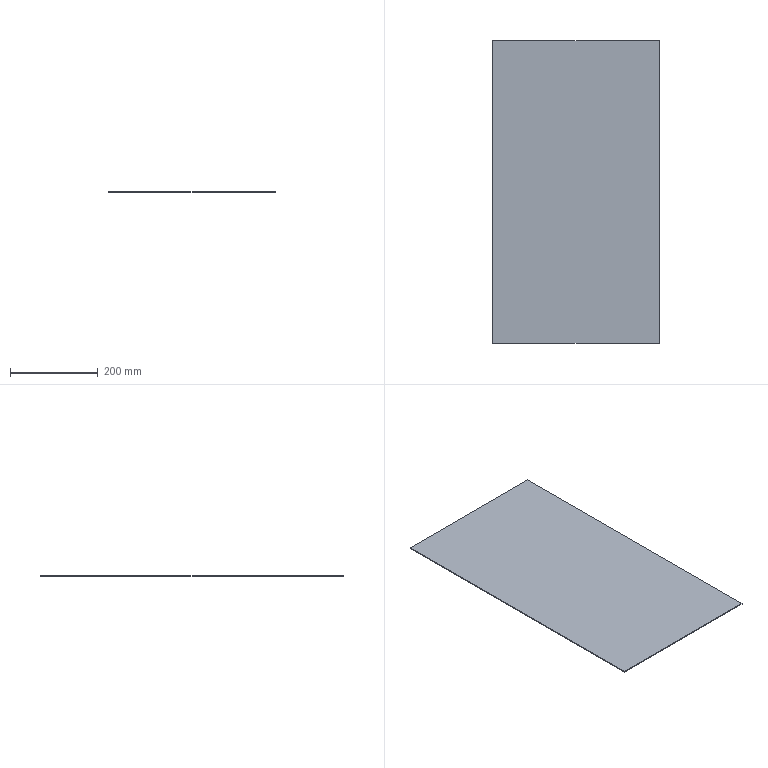Part | SolidWorks | features Extrusion 1 | 1 solid | 6 faces | box 380 x 690 x 2 mm | volume 524400 mm3 | plane 6
STEP:
#1=CARTESIAN_POINT('',(-337.882,161.453,0.));
#2=VERTEX_POINT('',#1);
#3=CARTESIAN_POINT('',(-337.882,-528.547,0.));
#4=VERTEX_POINT('',#3);
#5=CARTESIAN_POINT('',(-337.882,161.453,0.));
#6=DIRECTION('',(0.,-1.,0.));
#7=VECTOR('',#6,1000.);
#8=LINE('',#5,#7);
#9=EDGE_CURVE('',#2,#4,#8,.T.);
#10=ORIENTED_EDGE('',*,*,#9,.T.);
#11=CARTESIAN_POINT('',(-337.882,-528.547,2.));
#12=VERTEX_POINT('',#11);
#13=CARTESIAN_POINT('',(-337.882,-528.547,2.));
#14=DIRECTION('',(0.,0.,-1.));
#15=VECTOR('',#14,1000.);
#16=LINE('',#13,#15);
#17=EDGE_CURVE('',#12,#4,#16,.T.);
#18=ORIENTED_EDGE('',*,*,#17,.F.);
#19=CARTESIAN_POINT('',(-337.882,161.453,2.));
#20=VERTEX_POINT('',#19);
#21=CARTESIAN_POINT('',(-337.882,161.453,2.));
#22=DIRECTION('',(0.,-1.,0.));
#23=VECTOR('',#22,1000.);
#24=LINE('',#21,#23);
#25=EDGE_CURVE('',#20,#12,#24,.T.);
#26=ORIENTED_EDGE('',*,*,#25,.F.);
#27=CARTESIAN_POINT('',(-337.882,161.453,2.));
#28=DIRECTION('',(0.,0.,-1.));
#29=VECTOR('',#28,1000.);
#30=LINE('',#27,#29);
#31=EDGE_CURVE('',#20,#2,#30,.T.);
#32=ORIENTED_EDGE('',*,*,#31,.T.);
#33=EDGE_LOOP('',(#10,#18,#26,#32));
#34=FACE_OUTER_BOUND('',#33,.T.);
#35=CARTESIAN_POINT('',(-337.882,161.453,2.));
#36=DIRECTION('',(1.,0.,0.));
#37=DIRECTION('',(0.,1.,0.));
#38=AXIS2_PLACEMENT_3D('',#35,#36,#37);
#39=PLANE('',#38);
#40=ADVANCED_FACE('',(#34),#39,.F.);
#41=CARTESIAN_POINT('',(42.118,-528.547,0.));
#42=VERTEX_POINT('',#41);
#43=CARTESIAN_POINT('',(-337.882,-528.547,0.));
#44=DIRECTION('',(1.,0.,0.));
#45=VECTOR('',#44,1000.);
#46=LINE('',#43,#45);
#47=EDGE_CURVE('',#4,#42,#46,.T.);
#48=ORIENTED_EDGE('',*,*,#47,.T.);
#49=CARTESIAN_POINT('',(42.118,-528.547,2.));
#50=VERTEX_POINT('',#49);
#51=CARTESIAN_POINT('',(42.118,-528.547,2.));
#52=DIRECTION('',(0.,0.,-1.));
#53=VECTOR('',#52,1000.);
#54=LINE('',#51,#53);
#55=EDGE_CURVE('',#50,#42,#54,.T.);
#56=ORIENTED_EDGE('',*,*,#55,.F.);
#57=CARTESIAN_POINT('',(-337.882,-528.547,2.));
#58=DIRECTION('',(1.,0.,0.));
#59=VECTOR('',#58,1000.);
#60=LINE('',#57,#59);
#61=EDGE_CURVE('',#12,#50,#60,.T.);
#62=ORIENTED_EDGE('',*,*,#61,.F.);
#63=ORIENTED_EDGE('',*,*,#17,.T.);
#64=EDGE_LOOP('',(#48,#56,#62,#63));
#65=FACE_OUTER_BOUND('',#64,.T.);
#66=CARTESIAN_POINT('',(-337.882,-528.547,2.));
#67=DIRECTION('',(0.,1.,0.));
#68=DIRECTION('',(0.,0.,1.));
#69=AXIS2_PLACEMENT_3D('',#66,#67,#68);
#70=PLANE('',#69);
#71=ADVANCED_FACE('',(#65),#70,.F.);
#72=CARTESIAN_POINT('',(42.118,161.453,0.));
#73=VERTEX_POINT('',#72);
#74=CARTESIAN_POINT('',(42.118,161.453,0.));
#75=DIRECTION('',(0.,1.,0.));
#76=VECTOR('',#75,1000.);
#77=LINE('',#74,#76);
#78=EDGE_CURVE('',#42,#73,#77,.T.);
#79=ORIENTED_EDGE('',*,*,#78,.T.);
#80=CARTESIAN_POINT('',(42.118,161.453,2.));
#81=VERTEX_POINT('',#80);
#82=CARTESIAN_POINT('',(42.118,161.453,2.));
#83=DIRECTION('',(0.,0.,-1.));
#84=VECTOR('',#83,1000.);
#85=LINE('',#82,#84);
#86=EDGE_CURVE('',#81,#73,#85,.T.);
#87=ORIENTED_EDGE('',*,*,#86,.F.);
#88=CARTESIAN_POINT('',(42.118,161.453,2.));
#89=DIRECTION('',(0.,1.,0.));
#90=VECTOR('',#89,1000.);
#91=LINE('',#88,#90);
#92=EDGE_CURVE('',#50,#81,#91,.T.);
#93=ORIENTED_EDGE('',*,*,#92,.F.);
#94=ORIENTED_EDGE('',*,*,#55,.T.);
#95=EDGE_LOOP('',(#79,#87,#93,#94));
#96=FACE_OUTER_BOUND('',#95,.T.);
#97=CARTESIAN_POINT('',(42.118,161.453,2.));
#98=DIRECTION('',(-1.,0.,0.));
#99=DIRECTION('',(0.,-1.,0.));
#100=AXIS2_PLACEMENT_3D('',#97,#98,#99);
#101=PLANE('',#100);
#102=ADVANCED_FACE('',(#96),#101,.F.);
#103=CARTESIAN_POINT('',(-337.882,161.453,0.));
#104=DIRECTION('',(-1.,0.,0.));
#105=VECTOR('',#104,1000.);
#106=LINE('',#103,#105);
#107=EDGE_CURVE('',#73,#2,#106,.T.);
#108=ORIENTED_EDGE('',*,*,#107,.T.);
#109=ORIENTED_EDGE('',*,*,#31,.F.);
#110=CARTESIAN_POINT('',(-337.882,161.453,2.));
#111=DIRECTION('',(-1.,0.,0.));
#112=VECTOR('',#111,1000.);
#113=LINE('',#110,#112);
#114=EDGE_CURVE('',#81,#20,#113,.T.);
#115=ORIENTED_EDGE('',*,*,#114,.F.);
#116=ORIENTED_EDGE('',*,*,#86,.T.);
#117=EDGE_LOOP('',(#108,#109,#115,#116));
#118=FACE_OUTER_BOUND('',#117,.T.);
#119=CARTESIAN_POINT('',(-337.882,161.453,2.));
#120=DIRECTION('',(0.,-1.,0.));
#121=DIRECTION('',(0.,0.,-1.));
#122=AXIS2_PLACEMENT_3D('',#119,#120,#121);
#123=PLANE('',#122);
#124=ADVANCED_FACE('',(#118),#123,.F.);
#125=ORIENTED_EDGE('',*,*,#25,.T.);
#126=ORIENTED_EDGE('',*,*,#61,.T.);
#127=ORIENTED_EDGE('',*,*,#92,.T.);
#128=ORIENTED_EDGE('',*,*,#114,.T.);
#129=EDGE_LOOP('',(#125,#126,#127,#128));
#130=FACE_OUTER_BOUND('',#129,.T.);
#131=CARTESIAN_POINT('',(0.,0.,2.));
#132=DIRECTION('',(0.,0.,1.));
#133=DIRECTION('',(1.,0.,0.));
#134=AXIS2_PLACEMENT_3D('',#131,#132,#133);
#135=PLANE('',#134);
#136=ADVANCED_FACE('',(#130),#135,.T.);
#137=ORIENTED_EDGE('',*,*,#9,.F.);
#138=ORIENTED_EDGE('',*,*,#107,.F.);
#139=ORIENTED_EDGE('',*,*,#78,.F.);
#140=ORIENTED_EDGE('',*,*,#47,.F.);
#141=EDGE_LOOP('',(#137,#138,#139,#140));
#142=FACE_OUTER_BOUND('',#141,.T.);
#143=CARTESIAN_POINT('',(0.,0.,0.));
#144=DIRECTION('',(0.,0.,1.));
#145=DIRECTION('',(1.,0.,0.));
#146=AXIS2_PLACEMENT_3D('',#143,#144,#145);
#147=PLANE('',#146);
#148=ADVANCED_FACE('',(#142),#147,.F.);
#149=CLOSED_SHELL('',(#40,#71,#102,#124,#136,#148));
#150=MANIFOLD_SOLID_BREP('',#149);
#151=CARTESIAN_POINT('',(0.,0.,0.));
#152=DIRECTION('',(0.,0.,1.));
#153=DIRECTION('',(1.,0.,0.));
#154=AXIS2_PLACEMENT_3D('',#151,#152,#153);
#155=(LENGTH_UNIT()NAMED_UNIT(*)SI_UNIT(.MILLI.,.METRE.));
#156=UNCERTAINTY_MEASURE_WITH_UNIT(LENGTH_MEASURE(0.00001),#155,'','');
#157=(NAMED_UNIT(*)PLANE_ANGLE_UNIT()SI_UNIT($,.RADIAN.));
#158=(NAMED_UNIT(*)SI_UNIT($,.STERADIAN.)SOLID_ANGLE_UNIT());
#159=(GEOMETRIC_REPRESENTATION_CONTEXT(3)GLOBAL_UNCERTAINTY_ASSIGNED_CONTEXT((#156))GLOBAL_UNIT_ASSIGNED_CONTEXT((#155,#157,#158))REPRESENTATION_CONTEXT('',''));
#160=ADVANCED_BREP_SHAPE_REPRESENTATION('',(#150,#154),#159);